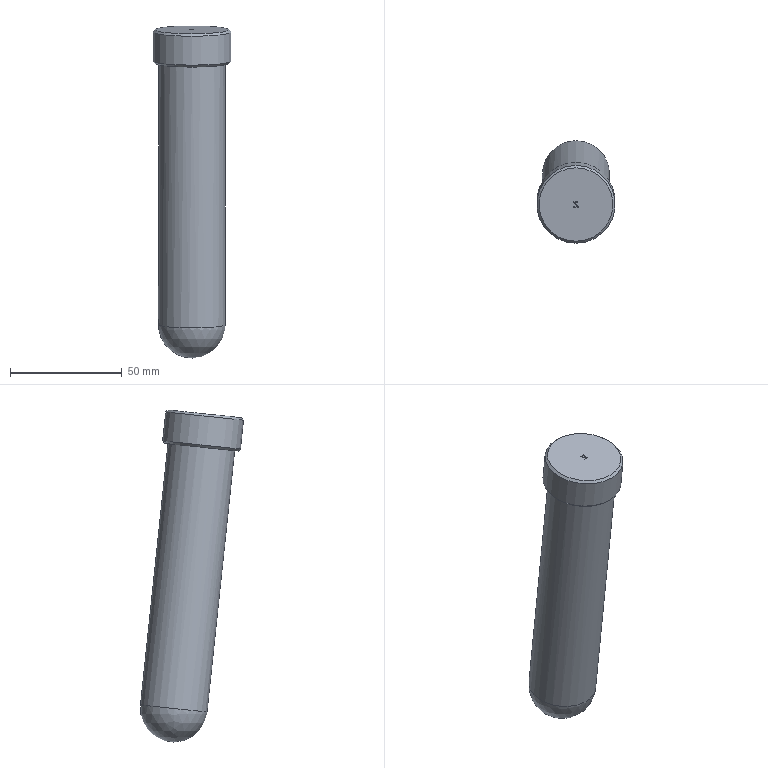Part | STEP file | solid 245 | 1 solid | 18 faces | box 35 x 46.15 x 148.499 mm | volume 104448 mm3 | plane 11 | cylinder 2 | other 2 | cone 2 | sphere 1 | commonest cylinder face diameters 30 x1 35 x1